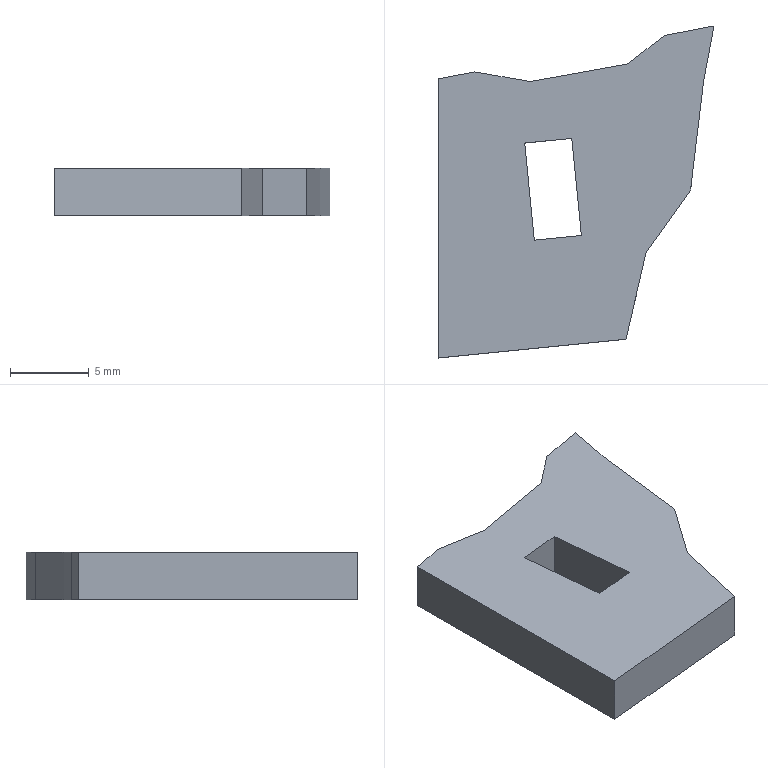Part | SolidWorks | features BaseBody 1 | 1 solid | 17 faces | box 17.508 x 21.063 x 3 mm | volume 743.607 mm3 | spline 10 | plane 7
STEP:
#1=CARTESIAN_POINT('',(4.82,4.837,-1.5));
#2=VERTEX_POINT('',#1);
#3=CARTESIAN_POINT('',(5.43,-1.324,-1.5));
#4=VERTEX_POINT('',#3);
#5=CARTESIAN_POINT('',(5.43,-1.324,-1.5));
#6=DIRECTION('',(0.09851,-0.9951,0.));
#7=VECTOR('',#6,1000.);
#8=LINE('',#5,#7);
#9=EDGE_CURVE('',#2,#4,#8,.T.);
#10=ORIENTED_EDGE('',*,*,#9,.F.);
#11=CARTESIAN_POINT('',(4.82,4.837,1.5));
#12=VERTEX_POINT('',#11);
#13=CARTESIAN_POINT('',(4.82,4.837,1.5));
#14=DIRECTION('',(0.,0.,-1.));
#15=VECTOR('',#14,1000.);
#16=LINE('',#13,#15);
#17=EDGE_CURVE('',#12,#2,#16,.T.);
#18=ORIENTED_EDGE('',*,*,#17,.F.);
#19=CARTESIAN_POINT('',(5.43,-1.324,1.5));
#20=VERTEX_POINT('',#19);
#21=CARTESIAN_POINT('',(5.43,-1.324,1.5));
#22=DIRECTION('',(0.09851,-0.9951,0.));
#23=VECTOR('',#22,1000.);
#24=LINE('',#21,#23);
#25=EDGE_CURVE('',#12,#20,#24,.T.);
#26=ORIENTED_EDGE('',*,*,#25,.T.);
#27=CARTESIAN_POINT('',(5.43,-1.324,1.5));
#28=DIRECTION('',(0.,0.,-1.));
#29=VECTOR('',#28,1000.);
#30=LINE('',#27,#29);
#31=EDGE_CURVE('',#20,#4,#30,.T.);
#32=ORIENTED_EDGE('',*,*,#31,.T.);
#33=EDGE_LOOP('',(#10,#18,#26,#32));
#34=FACE_OUTER_BOUND('',#33,.T.);
#35=CARTESIAN_POINT('',(5.43,-1.324,1.5));
#36=DIRECTION('',(0.9951,0.09851,0.));
#37=DIRECTION('',(0.,0.,-1.));
#38=AXIS2_PLACEMENT_3D('',#35,#36,#37);
#39=PLANE('',#38);
#40=ADVANCED_FACE('',(#34),#39,.T.);
#41=CARTESIAN_POINT('',(7.805,5.132,-1.5));
#42=VERTEX_POINT('',#41);
#43=CARTESIAN_POINT('',(7.805,5.132,-1.5));
#44=DIRECTION('',(-0.9951,-0.09851,0.));
#45=VECTOR('',#44,1000.);
#46=LINE('',#43,#45);
#47=EDGE_CURVE('',#42,#2,#46,.T.);
#48=ORIENTED_EDGE('',*,*,#47,.F.);
#49=CARTESIAN_POINT('',(7.805,5.132,1.5));
#50=VERTEX_POINT('',#49);
#51=CARTESIAN_POINT('',(7.805,5.132,1.5));
#52=DIRECTION('',(0.,0.,-1.));
#53=VECTOR('',#52,1000.);
#54=LINE('',#51,#53);
#55=EDGE_CURVE('',#50,#42,#54,.T.);
#56=ORIENTED_EDGE('',*,*,#55,.F.);
#57=CARTESIAN_POINT('',(7.805,5.132,1.5));
#58=DIRECTION('',(-0.9951,-0.09851,0.));
#59=VECTOR('',#58,1000.);
#60=LINE('',#57,#59);
#61=EDGE_CURVE('',#50,#12,#60,.T.);
#62=ORIENTED_EDGE('',*,*,#61,.T.);
#63=ORIENTED_EDGE('',*,*,#17,.T.);
#64=EDGE_LOOP('',(#48,#56,#62,#63));
#65=FACE_OUTER_BOUND('',#64,.T.);
#66=CARTESIAN_POINT('',(7.805,5.132,1.5));
#67=DIRECTION('',(0.09851,-0.9951,0.));
#68=DIRECTION('',(0.,0.,-1.));
#69=AXIS2_PLACEMENT_3D('',#66,#67,#68);
#70=PLANE('',#69);
#71=ADVANCED_FACE('',(#65),#70,.T.);
#72=CARTESIAN_POINT('',(8.415,-1.029,-1.5));
#73=VERTEX_POINT('',#72);
#74=CARTESIAN_POINT('',(8.415,-1.029,-1.5));
#75=DIRECTION('',(-0.09851,0.9951,0.));
#76=VECTOR('',#75,1000.);
#77=LINE('',#74,#76);
#78=EDGE_CURVE('',#73,#42,#77,.T.);
#79=ORIENTED_EDGE('',*,*,#78,.F.);
#80=CARTESIAN_POINT('',(8.415,-1.029,1.5));
#81=VERTEX_POINT('',#80);
#82=CARTESIAN_POINT('',(8.415,-1.029,1.5));
#83=DIRECTION('',(0.,0.,-1.));
#84=VECTOR('',#83,1000.);
#85=LINE('',#82,#84);
#86=EDGE_CURVE('',#81,#73,#85,.T.);
#87=ORIENTED_EDGE('',*,*,#86,.F.);
#88=CARTESIAN_POINT('',(8.415,-1.029,1.5));
#89=DIRECTION('',(-0.09851,0.9951,0.));
#90=VECTOR('',#89,1000.);
#91=LINE('',#88,#90);
#92=EDGE_CURVE('',#81,#50,#91,.T.);
#93=ORIENTED_EDGE('',*,*,#92,.T.);
#94=ORIENTED_EDGE('',*,*,#55,.T.);
#95=EDGE_LOOP('',(#79,#87,#93,#94));
#96=FACE_OUTER_BOUND('',#95,.T.);
#97=CARTESIAN_POINT('',(8.415,-1.029,1.5));
#98=DIRECTION('',(-0.9951,-0.09851,0.));
#99=DIRECTION('',(-0.09851,0.9951,0.));
#100=AXIS2_PLACEMENT_3D('',#97,#98,#99);
#101=PLANE('',#100);
#102=ADVANCED_FACE('',(#96),#101,.T.);
#103=CARTESIAN_POINT('',(8.415,-1.029,-1.5));
#104=DIRECTION('',(0.9951,0.09851,0.));
#105=VECTOR('',#104,1000.);
#106=LINE('',#103,#105);
#107=EDGE_CURVE('',#4,#73,#106,.T.);
#108=ORIENTED_EDGE('',*,*,#107,.F.);
#109=ORIENTED_EDGE('',*,*,#31,.F.);
#110=CARTESIAN_POINT('',(8.415,-1.029,1.5));
#111=DIRECTION('',(0.9951,0.09851,0.));
#112=VECTOR('',#111,1000.);
#113=LINE('',#110,#112);
#114=EDGE_CURVE('',#20,#81,#113,.T.);
#115=ORIENTED_EDGE('',*,*,#114,.T.);
#116=ORIENTED_EDGE('',*,*,#86,.T.);
#117=EDGE_LOOP('',(#108,#109,#115,#116));
#118=FACE_OUTER_BOUND('',#117,.T.);
#119=CARTESIAN_POINT('',(8.415,-1.029,1.5));
#120=DIRECTION('',(-0.09851,0.9951,0.));
#121=DIRECTION('',(0.,0.,1.));
#122=AXIS2_PLACEMENT_3D('',#119,#120,#121);
#123=PLANE('',#122);
#124=ADVANCED_FACE('',(#118),#123,.T.);
#125=CARTESIAN_POINT('',(5.187,8.742,-1.5));
#126=VERTEX_POINT('',#125);
#127=CARTESIAN_POINT('',(1.634,9.355,-1.5));
#128=VERTEX_POINT('',#127);
#129=CARTESIAN_POINT('',(5.187,8.742,-1.5));
#130=CARTESIAN_POINT('',(4.001,8.946,-1.5));
#131=CARTESIAN_POINT('',(2.817,9.149,-1.5));
#132=CARTESIAN_POINT('',(1.634,9.355,-1.5));
#133=B_SPLINE_CURVE_WITH_KNOTS('',3,(#129,#130,#131,#132),.UNSPECIFIED.,.F.,.F.,(4,4),(0.5238,0.5714),.UNSPECIFIED.);
#134=EDGE_CURVE('',#126,#128,#133,.T.);
#135=ORIENTED_EDGE('',*,*,#134,.T.);
#136=CARTESIAN_POINT('',(1.634,9.355,1.5));
#137=VERTEX_POINT('',#136);
#138=CARTESIAN_POINT('',(1.634,9.355,1.5));
#139=DIRECTION('',(0.,0.,-1.));
#140=VECTOR('',#139,1000.);
#141=LINE('',#138,#140);
#142=EDGE_CURVE('',#137,#128,#141,.T.);
#143=ORIENTED_EDGE('',*,*,#142,.F.);
#144=CARTESIAN_POINT('',(5.187,8.742,1.5));
#145=VERTEX_POINT('',#144);
#146=CARTESIAN_POINT('',(5.187,8.742,1.5));
#147=CARTESIAN_POINT('',(4.001,8.946,1.5));
#148=CARTESIAN_POINT('',(2.817,9.149,1.5));
#149=CARTESIAN_POINT('',(1.634,9.355,1.5));
#150=B_SPLINE_CURVE_WITH_KNOTS('',3,(#146,#147,#148,#149),.UNSPECIFIED.,.F.,.F.,(4,4),(0.5238,0.5714),.UNSPECIFIED.);
#151=EDGE_CURVE('',#145,#137,#150,.T.);
#152=ORIENTED_EDGE('',*,*,#151,.F.);
#153=CARTESIAN_POINT('',(5.187,8.742,1.5));
#154=DIRECTION('',(0.,0.,-1.));
#155=VECTOR('',#154,1000.);
#156=LINE('',#153,#155);
#157=EDGE_CURVE('',#145,#126,#156,.T.);
#158=ORIENTED_EDGE('',*,*,#157,.T.);
#159=EDGE_LOOP('',(#135,#143,#152,#158));
#160=FACE_OUTER_BOUND('',#159,.T.);
#161=CARTESIAN_POINT('',(5.187,8.742,1.5));
#162=CARTESIAN_POINT('',(5.187,8.742,-1.5));
#163=CARTESIAN_POINT('',(4.001,8.946,1.5));
#164=CARTESIAN_POINT('',(4.001,8.946,-1.5));
#165=CARTESIAN_POINT('',(2.817,9.149,1.5));
#166=CARTESIAN_POINT('',(2.817,9.149,-1.5));
#167=CARTESIAN_POINT('',(1.634,9.355,1.5));
#168=CARTESIAN_POINT('',(1.634,9.355,-1.5));
#169=B_SPLINE_SURFACE_WITH_KNOTS('',3,1,((#161,#162),(#163,#164),(#165,#166),(#167,#168)),.UNSPECIFIED.,.F.,.F.,.F.,(4,4),(2,2),(0.5238,0.5714),(0.,1.),.UNSPECIFIED.);
#170=ADVANCED_FACE('',(#160),#169,.F.);
#171=CARTESIAN_POINT('',(11.344,9.856,-1.5));
#172=VERTEX_POINT('',#171);
#173=CARTESIAN_POINT('',(11.344,9.856,-1.5));
#174=CARTESIAN_POINT('',(9.29,9.485,-1.5));
#175=CARTESIAN_POINT('',(7.239,9.113,-1.5));
#176=CARTESIAN_POINT('',(5.187,8.742,-1.5));
#177=B_SPLINE_CURVE_WITH_KNOTS('',3,(#173,#174,#175,#176),.UNSPECIFIED.,.F.,.F.,(4,4),(0.5714,0.619),.UNSPECIFIED.);
#178=EDGE_CURVE('',#172,#126,#177,.T.);
#179=ORIENTED_EDGE('',*,*,#178,.T.);
#180=ORIENTED_EDGE('',*,*,#157,.F.);
#181=CARTESIAN_POINT('',(11.344,9.856,1.5));
#182=VERTEX_POINT('',#181);
#183=CARTESIAN_POINT('',(11.344,9.856,1.5));
#184=CARTESIAN_POINT('',(9.29,9.485,1.5));
#185=CARTESIAN_POINT('',(7.239,9.113,1.5));
#186=CARTESIAN_POINT('',(5.187,8.742,1.5));
#187=B_SPLINE_CURVE_WITH_KNOTS('',3,(#183,#184,#185,#186),.UNSPECIFIED.,.F.,.F.,(4,4),(0.5714,0.619),.UNSPECIFIED.);
#188=EDGE_CURVE('',#182,#145,#187,.T.);
#189=ORIENTED_EDGE('',*,*,#188,.F.);
#190=CARTESIAN_POINT('',(11.344,9.856,1.5));
#191=DIRECTION('',(0.,0.,-1.));
#192=VECTOR('',#191,1000.);
#193=LINE('',#190,#192);
#194=EDGE_CURVE('',#182,#172,#193,.T.);
#195=ORIENTED_EDGE('',*,*,#194,.T.);
#196=EDGE_LOOP('',(#179,#180,#189,#195));
#197=FACE_OUTER_BOUND('',#196,.T.);
#198=CARTESIAN_POINT('',(11.344,9.856,1.5));
#199=CARTESIAN_POINT('',(11.344,9.856,-1.5));
#200=CARTESIAN_POINT('',(9.29,9.485,1.5));
#201=CARTESIAN_POINT('',(9.29,9.485,-1.5));
#202=CARTESIAN_POINT('',(7.239,9.113,1.5));
#203=CARTESIAN_POINT('',(7.239,9.113,-1.5));
#204=CARTESIAN_POINT('',(5.187,8.742,1.5));
#205=CARTESIAN_POINT('',(5.187,8.742,-1.5));
#206=B_SPLINE_SURFACE_WITH_KNOTS('',3,1,((#198,#199),(#200,#201),(#202,#203),(#204,#205)),.UNSPECIFIED.,.F.,.F.,.F.,(4,4),(2,2),(0.5714,0.619),(0.,1.),.UNSPECIFIED.);
#207=ADVANCED_FACE('',(#197),#206,.F.);
#208=CARTESIAN_POINT('',(13.682,11.663,-1.5));
#209=VERTEX_POINT('',#208);
#210=CARTESIAN_POINT('',(13.682,11.663,-1.5));
#211=CARTESIAN_POINT('',(12.903,11.062,-1.5));
#212=CARTESIAN_POINT('',(12.123,10.459,-1.5));
#213=CARTESIAN_POINT('',(11.344,9.856,-1.5));
#214=B_SPLINE_CURVE_WITH_KNOTS('',3,(#210,#211,#212,#213),.UNSPECIFIED.,.F.,.F.,(4,4),(0.619,0.6667),.UNSPECIFIED.);
#215=EDGE_CURVE('',#209,#172,#214,.T.);
#216=ORIENTED_EDGE('',*,*,#215,.T.);
#217=ORIENTED_EDGE('',*,*,#194,.F.);
#218=CARTESIAN_POINT('',(13.682,11.663,1.5));
#219=VERTEX_POINT('',#218);
#220=CARTESIAN_POINT('',(13.682,11.663,1.5));
#221=CARTESIAN_POINT('',(12.903,11.062,1.5));
#222=CARTESIAN_POINT('',(12.123,10.459,1.5));
#223=CARTESIAN_POINT('',(11.344,9.856,1.5));
#224=B_SPLINE_CURVE_WITH_KNOTS('',3,(#220,#221,#222,#223),.UNSPECIFIED.,.F.,.F.,(4,4),(0.619,0.6667),.UNSPECIFIED.);
#225=EDGE_CURVE('',#219,#182,#224,.T.);
#226=ORIENTED_EDGE('',*,*,#225,.F.);
#227=CARTESIAN_POINT('',(13.682,11.663,1.5));
#228=DIRECTION('',(0.,0.,-1.));
#229=VECTOR('',#228,1000.);
#230=LINE('',#227,#229);
#231=EDGE_CURVE('',#219,#209,#230,.T.);
#232=ORIENTED_EDGE('',*,*,#231,.T.);
#233=EDGE_LOOP('',(#216,#217,#226,#232));
#234=FACE_OUTER_BOUND('',#233,.T.);
#235=CARTESIAN_POINT('',(13.682,11.663,1.5));
#236=CARTESIAN_POINT('',(13.682,11.663,-1.5));
#237=CARTESIAN_POINT('',(12.903,11.062,1.5));
#238=CARTESIAN_POINT('',(12.903,11.062,-1.5));
#239=CARTESIAN_POINT('',(12.123,10.459,1.5));
#240=CARTESIAN_POINT('',(12.123,10.459,-1.5));
#241=CARTESIAN_POINT('',(11.344,9.856,1.5));
#242=CARTESIAN_POINT('',(11.344,9.856,-1.5));
#243=B_SPLINE_SURFACE_WITH_KNOTS('',3,1,((#235,#236),(#237,#238),(#239,#240),(#241,#242)),.UNSPECIFIED.,.F.,.F.,.F.,(4,4),(2,2),(0.619,0.6667),(0.,1.),.UNSPECIFIED.);
#244=ADVANCED_FACE('',(#234),#243,.F.);
#245=CARTESIAN_POINT('',(16.827,12.266,-1.5));
#246=VERTEX_POINT('',#245);
#247=CARTESIAN_POINT('',(16.827,12.266,-1.5));
#248=CARTESIAN_POINT('',(15.779,12.065,-1.5));
#249=CARTESIAN_POINT('',(14.73,11.862,-1.5));
#250=CARTESIAN_POINT('',(13.682,11.663,-1.5));
#251=B_SPLINE_CURVE_WITH_KNOTS('',3,(#247,#248,#249,#250),.UNSPECIFIED.,.F.,.F.,(4,4),(0.6667,0.7143),.UNSPECIFIED.);
#252=EDGE_CURVE('',#246,#209,#251,.T.);
#253=ORIENTED_EDGE('',*,*,#252,.T.);
#254=ORIENTED_EDGE('',*,*,#231,.F.);
#255=CARTESIAN_POINT('',(16.827,12.266,1.5));
#256=VERTEX_POINT('',#255);
#257=CARTESIAN_POINT('',(16.827,12.266,1.5));
#258=CARTESIAN_POINT('',(15.779,12.065,1.5));
#259=CARTESIAN_POINT('',(14.73,11.862,1.5));
#260=CARTESIAN_POINT('',(13.682,11.663,1.5));
#261=B_SPLINE_CURVE_WITH_KNOTS('',3,(#257,#258,#259,#260),.UNSPECIFIED.,.F.,.F.,(4,4),(0.6667,0.7143),.UNSPECIFIED.);
#262=EDGE_CURVE('',#256,#219,#261,.T.);
#263=ORIENTED_EDGE('',*,*,#262,.F.);
#264=CARTESIAN_POINT('',(16.827,12.266,1.5));
#265=DIRECTION('',(0.,0.,-1.));
#266=VECTOR('',#265,1000.);
#267=LINE('',#264,#266);
#268=EDGE_CURVE('',#256,#246,#267,.T.);
#269=ORIENTED_EDGE('',*,*,#268,.T.);
#270=EDGE_LOOP('',(#253,#254,#263,#269));
#271=FACE_OUTER_BOUND('',#270,.T.);
#272=CARTESIAN_POINT('',(16.827,12.266,1.5));
#273=CARTESIAN_POINT('',(16.827,12.266,-1.5));
#274=CARTESIAN_POINT('',(15.779,12.065,1.5));
#275=CARTESIAN_POINT('',(15.779,12.065,-1.5));
#276=CARTESIAN_POINT('',(14.73,11.862,1.5));
#277=CARTESIAN_POINT('',(14.73,11.862,-1.5));
#278=CARTESIAN_POINT('',(13.682,11.663,1.5));
#279=CARTESIAN_POINT('',(13.682,11.663,-1.5));
#280=B_SPLINE_SURFACE_WITH_KNOTS('',3,1,((#272,#273),(#274,#275),(#276,#277),(#278,#279)),.UNSPECIFIED.,.F.,.F.,.F.,(4,4),(2,2),(0.6667,0.7143),(0.,1.),.UNSPECIFIED.);
#281=ADVANCED_FACE('',(#271),#280,.F.);
#282=CARTESIAN_POINT('',(16.177,8.839,-1.5));
#283=VERTEX_POINT('',#282);
#284=CARTESIAN_POINT('',(16.177,8.839,-1.5));
#285=CARTESIAN_POINT('',(16.394,9.981,-1.5));
#286=CARTESIAN_POINT('',(16.612,11.122,-1.5));
#287=CARTESIAN_POINT('',(16.827,12.266,-1.5));
#288=B_SPLINE_CURVE_WITH_KNOTS('',3,(#284,#285,#286,#287),.UNSPECIFIED.,.F.,.F.,(4,4),(0.7143,0.7619),.UNSPECIFIED.);
#289=EDGE_CURVE('',#283,#246,#288,.T.);
#290=ORIENTED_EDGE('',*,*,#289,.T.);
#291=ORIENTED_EDGE('',*,*,#268,.F.);
#292=CARTESIAN_POINT('',(16.177,8.839,1.5));
#293=VERTEX_POINT('',#292);
#294=CARTESIAN_POINT('',(16.177,8.839,1.5));
#295=CARTESIAN_POINT('',(16.394,9.981,1.5));
#296=CARTESIAN_POINT('',(16.612,11.122,1.5));
#297=CARTESIAN_POINT('',(16.827,12.266,1.5));
#298=B_SPLINE_CURVE_WITH_KNOTS('',3,(#294,#295,#296,#297),.UNSPECIFIED.,.F.,.F.,(4,4),(0.7143,0.7619),.UNSPECIFIED.);
#299=EDGE_CURVE('',#293,#256,#298,.T.);
#300=ORIENTED_EDGE('',*,*,#299,.F.);
#301=CARTESIAN_POINT('',(16.177,8.839,1.5));
#302=DIRECTION('',(0.,0.,-1.));
#303=VECTOR('',#302,1000.);
#304=LINE('',#301,#303);
#305=EDGE_CURVE('',#293,#283,#304,.T.);
#306=ORIENTED_EDGE('',*,*,#305,.T.);
#307=EDGE_LOOP('',(#290,#291,#300,#306));
#308=FACE_OUTER_BOUND('',#307,.T.);
#309=CARTESIAN_POINT('',(16.177,8.839,1.5));
#310=CARTESIAN_POINT('',(16.177,8.839,-1.5));
#311=CARTESIAN_POINT('',(16.394,9.981,1.5));
#312=CARTESIAN_POINT('',(16.394,9.981,-1.5));
#313=CARTESIAN_POINT('',(16.612,11.122,1.5));
#314=CARTESIAN_POINT('',(16.612,11.122,-1.5));
#315=CARTESIAN_POINT('',(16.827,12.266,1.5));
#316=CARTESIAN_POINT('',(16.827,12.266,-1.5));
#317=B_SPLINE_SURFACE_WITH_KNOTS('',3,1,((#309,#310),(#311,#312),(#313,#314),(#315,#316)),.UNSPECIFIED.,.F.,.F.,.F.,(4,4),(2,2),(0.7143,0.7619),(0.,1.),.UNSPECIFIED.);
#318=ADVANCED_FACE('',(#308),#317,.F.);
#319=CARTESIAN_POINT('',(15.344,1.858,-1.5));
#320=VERTEX_POINT('',#319);
#321=CARTESIAN_POINT('',(15.344,1.858,-1.5));
#322=CARTESIAN_POINT('',(15.623,4.185,-1.5));
#323=CARTESIAN_POINT('',(15.902,6.512,-1.5));
#324=CARTESIAN_POINT('',(16.177,8.839,-1.5));
#325=B_SPLINE_CURVE_WITH_KNOTS('',3,(#321,#322,#323,#324),.UNSPECIFIED.,.F.,.F.,(4,4),(0.7619,0.8095),.UNSPECIFIED.);
#326=EDGE_CURVE('',#320,#283,#325,.T.);
#327=ORIENTED_EDGE('',*,*,#326,.T.);
#328=ORIENTED_EDGE('',*,*,#305,.F.);
#329=CARTESIAN_POINT('',(15.344,1.858,1.5));
#330=VERTEX_POINT('',#329);
#331=CARTESIAN_POINT('',(15.344,1.858,1.5));
#332=CARTESIAN_POINT('',(15.623,4.185,1.5));
#333=CARTESIAN_POINT('',(15.902,6.512,1.5));
#334=CARTESIAN_POINT('',(16.177,8.839,1.5));
#335=B_SPLINE_CURVE_WITH_KNOTS('',3,(#331,#332,#333,#334),.UNSPECIFIED.,.F.,.F.,(4,4),(0.7619,0.8095),.UNSPECIFIED.);
#336=EDGE_CURVE('',#330,#293,#335,.T.);
#337=ORIENTED_EDGE('',*,*,#336,.F.);
#338=CARTESIAN_POINT('',(15.344,1.858,1.5));
#339=DIRECTION('',(0.,0.,-1.));
#340=VECTOR('',#339,1000.);
#341=LINE('',#338,#340);
#342=EDGE_CURVE('',#330,#320,#341,.T.);
#343=ORIENTED_EDGE('',*,*,#342,.T.);
#344=EDGE_LOOP('',(#327,#328,#337,#343));
#345=FACE_OUTER_BOUND('',#344,.T.);
#346=CARTESIAN_POINT('',(15.344,1.858,1.5));
#347=CARTESIAN_POINT('',(15.344,1.858,-1.5));
#348=CARTESIAN_POINT('',(15.623,4.185,1.5));
#349=CARTESIAN_POINT('',(15.623,4.185,-1.5));
#350=CARTESIAN_POINT('',(15.902,6.512,1.5));
#351=CARTESIAN_POINT('',(15.902,6.512,-1.5));
#352=CARTESIAN_POINT('',(16.177,8.839,1.5));
#353=CARTESIAN_POINT('',(16.177,8.839,-1.5));
#354=B_SPLINE_SURFACE_WITH_KNOTS('',3,1,((#346,#347),(#348,#349),(#350,#351),(#352,#353)),.UNSPECIFIED.,.F.,.F.,.F.,(4,4),(2,2),(0.7619,0.8095),(0.,1.),.UNSPECIFIED.);
#355=ADVANCED_FACE('',(#345),#354,.F.);
#356=CARTESIAN_POINT('',(12.521,-2.113,-1.5));
#357=VERTEX_POINT('',#356);
#358=CARTESIAN_POINT('',(12.521,-2.113,-1.5));
#359=CARTESIAN_POINT('',(13.464,-0.7892,-1.5));
#360=CARTESIAN_POINT('',(14.405,0.5349,-1.5));
#361=CARTESIAN_POINT('',(15.344,1.858,-1.5));
#362=B_SPLINE_CURVE_WITH_KNOTS('',3,(#358,#359,#360,#361),.UNSPECIFIED.,.F.,.F.,(4,4),(0.8095,0.8571),.UNSPECIFIED.);
#363=EDGE_CURVE('',#357,#320,#362,.T.);
#364=ORIENTED_EDGE('',*,*,#363,.T.);
#365=ORIENTED_EDGE('',*,*,#342,.F.);
#366=CARTESIAN_POINT('',(12.521,-2.113,1.5));
#367=VERTEX_POINT('',#366);
#368=CARTESIAN_POINT('',(12.521,-2.113,1.5));
#369=CARTESIAN_POINT('',(13.464,-0.7892,1.5));
#370=CARTESIAN_POINT('',(14.405,0.5349,1.5));
#371=CARTESIAN_POINT('',(15.344,1.858,1.5));
#372=B_SPLINE_CURVE_WITH_KNOTS('',3,(#368,#369,#370,#371),.UNSPECIFIED.,.F.,.F.,(4,4),(0.8095,0.8571),.UNSPECIFIED.);
#373=EDGE_CURVE('',#367,#330,#372,.T.);
#374=ORIENTED_EDGE('',*,*,#373,.F.);
#375=CARTESIAN_POINT('',(12.521,-2.113,1.5));
#376=DIRECTION('',(0.,0.,-1.));
#377=VECTOR('',#376,1000.);
#378=LINE('',#375,#377);
#379=EDGE_CURVE('',#367,#357,#378,.T.);
#380=ORIENTED_EDGE('',*,*,#379,.T.);
#381=EDGE_LOOP('',(#364,#365,#374,#380));
#382=FACE_OUTER_BOUND('',#381,.T.);
#383=CARTESIAN_POINT('',(12.521,-2.113,1.5));
#384=CARTESIAN_POINT('',(12.521,-2.113,-1.5));
#385=CARTESIAN_POINT('',(13.464,-0.7892,1.5));
#386=CARTESIAN_POINT('',(13.464,-0.7892,-1.5));
#387=CARTESIAN_POINT('',(14.405,0.5349,1.5));
#388=CARTESIAN_POINT('',(14.405,0.5349,-1.5));
#389=CARTESIAN_POINT('',(15.344,1.858,1.5));
#390=CARTESIAN_POINT('',(15.344,1.858,-1.5));
#391=B_SPLINE_SURFACE_WITH_KNOTS('',3,1,((#383,#384),(#385,#386),(#387,#388),(#389,#390)),.UNSPECIFIED.,.F.,.F.,.F.,(4,4),(2,2),(0.8095,0.8571),(0.,1.),.UNSPECIFIED.);
#392=ADVANCED_FACE('',(#382),#391,.F.);
#393=CARTESIAN_POINT('',(11.243,-7.615,-1.5));
#394=VERTEX_POINT('',#393);
#395=CARTESIAN_POINT('',(11.243,-7.615,-1.5));
#396=CARTESIAN_POINT('',(11.669,-5.78,-1.5));
#397=CARTESIAN_POINT('',(12.097,-3.948,-1.5));
#398=CARTESIAN_POINT('',(12.521,-2.113,-1.5));
#399=B_SPLINE_CURVE_WITH_KNOTS('',3,(#395,#396,#397,#398),.UNSPECIFIED.,.F.,.F.,(4,4),(0.8571,0.9048),.UNSPECIFIED.);
#400=EDGE_CURVE('',#394,#357,#399,.T.);
#401=ORIENTED_EDGE('',*,*,#400,.T.);
#402=ORIENTED_EDGE('',*,*,#379,.F.);
#403=CARTESIAN_POINT('',(11.243,-7.615,1.5));
#404=VERTEX_POINT('',#403);
#405=CARTESIAN_POINT('',(11.243,-7.615,1.5));
#406=CARTESIAN_POINT('',(11.669,-5.78,1.5));
#407=CARTESIAN_POINT('',(12.097,-3.948,1.5));
#408=CARTESIAN_POINT('',(12.521,-2.113,1.5));
#409=B_SPLINE_CURVE_WITH_KNOTS('',3,(#405,#406,#407,#408),.UNSPECIFIED.,.F.,.F.,(4,4),(0.8571,0.9048),.UNSPECIFIED.);
#410=EDGE_CURVE('',#404,#367,#409,.T.);
#411=ORIENTED_EDGE('',*,*,#410,.F.);
#412=CARTESIAN_POINT('',(11.243,-7.615,1.5));
#413=DIRECTION('',(0.,0.,-1.));
#414=VECTOR('',#413,1000.);
#415=LINE('',#412,#414);
#416=EDGE_CURVE('',#404,#394,#415,.T.);
#417=ORIENTED_EDGE('',*,*,#416,.T.);
#418=EDGE_LOOP('',(#401,#402,#411,#417));
#419=FACE_OUTER_BOUND('',#418,.T.);
#420=CARTESIAN_POINT('',(11.243,-7.615,1.5));
#421=CARTESIAN_POINT('',(11.243,-7.615,-1.5));
#422=CARTESIAN_POINT('',(11.669,-5.78,1.5));
#423=CARTESIAN_POINT('',(11.669,-5.78,-1.5));
#424=CARTESIAN_POINT('',(12.097,-3.948,1.5));
#425=CARTESIAN_POINT('',(12.097,-3.948,-1.5));
#426=CARTESIAN_POINT('',(12.521,-2.113,1.5));
#427=CARTESIAN_POINT('',(12.521,-2.113,-1.5));
#428=B_SPLINE_SURFACE_WITH_KNOTS('',3,1,((#420,#421),(#422,#423),(#424,#425),(#426,#427)),.UNSPECIFIED.,.F.,.F.,.F.,(4,4),(2,2),(0.8571,0.9048),(0.,1.),.UNSPECIFIED.);
#429=ADVANCED_FACE('',(#419),#428,.F.);
#430=CARTESIAN_POINT('',(-0.6806,-8.797,-1.5));
#431=VERTEX_POINT('',#430);
#432=CARTESIAN_POINT('',(-0.6806,-8.797,-1.5));
#433=CARTESIAN_POINT('',(3.294,-8.402,-1.5));
#434=CARTESIAN_POINT('',(7.27,-8.009,-1.5));
#435=CARTESIAN_POINT('',(11.243,-7.615,-1.5));
#436=B_SPLINE_CURVE_WITH_KNOTS('',3,(#432,#433,#434,#435),.UNSPECIFIED.,.F.,.F.,(4,4),(0.9048,1.),.UNSPECIFIED.);
#437=EDGE_CURVE('',#431,#394,#436,.T.);
#438=ORIENTED_EDGE('',*,*,#437,.T.);
#439=ORIENTED_EDGE('',*,*,#416,.F.);
#440=CARTESIAN_POINT('',(-0.6806,-8.797,1.5));
#441=VERTEX_POINT('',#440);
#442=CARTESIAN_POINT('',(-0.6806,-8.797,1.5));
#443=CARTESIAN_POINT('',(3.294,-8.402,1.5));
#444=CARTESIAN_POINT('',(7.27,-8.009,1.5));
#445=CARTESIAN_POINT('',(11.243,-7.615,1.5));
#446=B_SPLINE_CURVE_WITH_KNOTS('',3,(#442,#443,#444,#445),.UNSPECIFIED.,.F.,.F.,(4,4),(0.9048,1.),.UNSPECIFIED.);
#447=EDGE_CURVE('',#441,#404,#446,.T.);
#448=ORIENTED_EDGE('',*,*,#447,.F.);
#449=CARTESIAN_POINT('',(-0.6806,-8.797,1.5));
#450=DIRECTION('',(0.,0.,-1.));
#451=VECTOR('',#450,1000.);
#452=LINE('',#449,#451);
#453=EDGE_CURVE('',#441,#431,#452,.T.);
#454=ORIENTED_EDGE('',*,*,#453,.T.);
#455=EDGE_LOOP('',(#438,#439,#448,#454));
#456=FACE_OUTER_BOUND('',#455,.T.);
#457=CARTESIAN_POINT('',(-0.6806,-8.797,1.5));
#458=CARTESIAN_POINT('',(-0.6806,-8.797,-1.5));
#459=CARTESIAN_POINT('',(3.294,-8.402,1.5));
#460=CARTESIAN_POINT('',(3.294,-8.402,-1.5));
#461=CARTESIAN_POINT('',(7.27,-8.009,1.5));
#462=CARTESIAN_POINT('',(7.27,-8.009,-1.5));
#463=CARTESIAN_POINT('',(11.243,-7.615,1.5));
#464=CARTESIAN_POINT('',(11.243,-7.615,-1.5));
#465=B_SPLINE_SURFACE_WITH_KNOTS('',3,1,((#457,#458),(#459,#460),(#461,#462),(#463,#464)),.UNSPECIFIED.,.F.,.F.,.F.,(4,4),(2,2),(0.9048,1.),(0.,1.),.UNSPECIFIED.);
#466=ADVANCED_FACE('',(#456),#465,.F.);
#467=CARTESIAN_POINT('',(-0.6806,8.91,-1.5));
#468=VERTEX_POINT('',#467);
#469=CARTESIAN_POINT('',(-0.6806,8.91,-1.5));
#470=DIRECTION('',(0.,-1.,0.));
#471=VECTOR('',#470,1000.);
#472=LINE('',#469,#471);
#473=EDGE_CURVE('',#468,#431,#472,.T.);
#474=ORIENTED_EDGE('',*,*,#473,.T.);
#475=ORIENTED_EDGE('',*,*,#453,.F.);
#476=CARTESIAN_POINT('',(-0.6806,8.91,1.5));
#477=VERTEX_POINT('',#476);
#478=CARTESIAN_POINT('',(-0.6806,8.91,1.5));
#479=DIRECTION('',(0.,-1.,0.));
#480=VECTOR('',#479,1000.);
#481=LINE('',#478,#480);
#482=EDGE_CURVE('',#477,#441,#481,.T.);
#483=ORIENTED_EDGE('',*,*,#482,.F.);
#484=CARTESIAN_POINT('',(-0.6806,8.91,1.5));
#485=DIRECTION('',(0.,0.,-1.));
#486=VECTOR('',#485,1000.);
#487=LINE('',#484,#486);
#488=EDGE_CURVE('',#477,#468,#487,.T.);
#489=ORIENTED_EDGE('',*,*,#488,.T.);
#490=EDGE_LOOP('',(#474,#475,#483,#489));
#491=FACE_OUTER_BOUND('',#490,.T.);
#492=CARTESIAN_POINT('',(-0.6806,8.91,1.5));
#493=DIRECTION('',(1.,0.,0.));
#494=DIRECTION('',(0.,1.,0.));
#495=AXIS2_PLACEMENT_3D('',#492,#493,#494);
#496=PLANE('',#495);
#497=ADVANCED_FACE('',(#491),#496,.F.);
#498=CARTESIAN_POINT('',(1.634,9.355,-1.5));
#499=CARTESIAN_POINT('',(0.863,9.206,-1.5));
#500=CARTESIAN_POINT('',(0.09044,9.059,-1.5));
#501=CARTESIAN_POINT('',(-0.6806,8.91,-1.5));
#502=B_SPLINE_CURVE_WITH_KNOTS('',3,(#498,#499,#500,#501),.UNSPECIFIED.,.F.,.F.,(4,4),(0.4762,0.5238),.UNSPECIFIED.);
#503=EDGE_CURVE('',#128,#468,#502,.T.);
#504=ORIENTED_EDGE('',*,*,#503,.T.);
#505=ORIENTED_EDGE('',*,*,#488,.F.);
#506=CARTESIAN_POINT('',(1.634,9.355,1.5));
#507=CARTESIAN_POINT('',(0.863,9.206,1.5));
#508=CARTESIAN_POINT('',(0.09044,9.059,1.5));
#509=CARTESIAN_POINT('',(-0.6806,8.91,1.5));
#510=B_SPLINE_CURVE_WITH_KNOTS('',3,(#506,#507,#508,#509),.UNSPECIFIED.,.F.,.F.,(4,4),(0.4762,0.5238),.UNSPECIFIED.);
#511=EDGE_CURVE('',#137,#477,#510,.T.);
#512=ORIENTED_EDGE('',*,*,#511,.F.);
#513=ORIENTED_EDGE('',*,*,#142,.T.);
#514=EDGE_LOOP('',(#504,#505,#512,#513));
#515=FACE_OUTER_BOUND('',#514,.T.);
#516=CARTESIAN_POINT('',(1.634,9.355,1.5));
#517=CARTESIAN_POINT('',(1.634,9.355,-1.5));
#518=CARTESIAN_POINT('',(0.863,9.206,1.5));
#519=CARTESIAN_POINT('',(0.863,9.206,-1.5));
#520=CARTESIAN_POINT('',(0.09044,9.059,1.5));
#521=CARTESIAN_POINT('',(0.09044,9.059,-1.5));
#522=CARTESIAN_POINT('',(-0.6806,8.91,1.5));
#523=CARTESIAN_POINT('',(-0.6806,8.91,-1.5));
#524=B_SPLINE_SURFACE_WITH_KNOTS('',3,1,((#516,#517),(#518,#519),(#520,#521),(#522,#523)),.UNSPECIFIED.,.F.,.F.,.F.,(4,4),(2,2),(0.4762,0.5238),(0.,1.),.UNSPECIFIED.);
#525=ADVANCED_FACE('',(#515),#524,.F.);
#526=ORIENTED_EDGE('',*,*,#107,.T.);
#527=ORIENTED_EDGE('',*,*,#78,.T.);
#528=ORIENTED_EDGE('',*,*,#47,.T.);
#529=ORIENTED_EDGE('',*,*,#9,.T.);
#530=EDGE_LOOP('',(#526,#527,#528,#529));
#531=FACE_BOUND('',#530,.T.);
#532=ORIENTED_EDGE('',*,*,#503,.F.);
#533=ORIENTED_EDGE('',*,*,#134,.F.);
#534=ORIENTED_EDGE('',*,*,#178,.F.);
#535=ORIENTED_EDGE('',*,*,#215,.F.);
#536=ORIENTED_EDGE('',*,*,#252,.F.);
#537=ORIENTED_EDGE('',*,*,#289,.F.);
#538=ORIENTED_EDGE('',*,*,#326,.F.);
#539=ORIENTED_EDGE('',*,*,#363,.F.);
#540=ORIENTED_EDGE('',*,*,#400,.F.);
#541=ORIENTED_EDGE('',*,*,#437,.F.);
#542=ORIENTED_EDGE('',*,*,#473,.F.);
#543=EDGE_LOOP('',(#532,#533,#534,#535,#536,#537,#538,#539,#540,#541,#542));
#544=FACE_OUTER_BOUND('',#543,.T.);
#545=CARTESIAN_POINT('',(0.4767,9.133,-1.5));
#546=DIRECTION('',(0.,0.,1.));
#547=DIRECTION('',(1.,0.,0.));
#548=AXIS2_PLACEMENT_3D('',#545,#546,#547);
#549=PLANE('',#548);
#550=ADVANCED_FACE('',(#531,#544),#549,.F.);
#551=ORIENTED_EDGE('',*,*,#92,.F.);
#552=ORIENTED_EDGE('',*,*,#114,.F.);
#553=ORIENTED_EDGE('',*,*,#25,.F.);
#554=ORIENTED_EDGE('',*,*,#61,.F.);
#555=EDGE_LOOP('',(#551,#552,#553,#554));
#556=FACE_BOUND('',#555,.T.);
#557=ORIENTED_EDGE('',*,*,#511,.T.);
#558=ORIENTED_EDGE('',*,*,#482,.T.);
#559=ORIENTED_EDGE('',*,*,#447,.T.);
#560=ORIENTED_EDGE('',*,*,#410,.T.);
#561=ORIENTED_EDGE('',*,*,#373,.T.);
#562=ORIENTED_EDGE('',*,*,#336,.T.);
#563=ORIENTED_EDGE('',*,*,#299,.T.);
#564=ORIENTED_EDGE('',*,*,#262,.T.);
#565=ORIENTED_EDGE('',*,*,#225,.T.);
#566=ORIENTED_EDGE('',*,*,#188,.T.);
#567=ORIENTED_EDGE('',*,*,#151,.T.);
#568=EDGE_LOOP('',(#557,#558,#559,#560,#561,#562,#563,#564,#565,#566,#567));
#569=FACE_OUTER_BOUND('',#568,.T.);
#570=CARTESIAN_POINT('',(0.4767,9.133,1.5));
#571=DIRECTION('',(0.,0.,1.));
#572=DIRECTION('',(1.,0.,0.));
#573=AXIS2_PLACEMENT_3D('',#570,#571,#572);
#574=PLANE('',#573);
#575=ADVANCED_FACE('',(#556,#569),#574,.T.);
#576=CLOSED_SHELL('',(#40,#71,#102,#124,#170,#207,#244,#281,#318,#355,#392,#429,#466,#497,#525,#550,#575));
#577=MANIFOLD_SOLID_BREP('',#576);
#578=CARTESIAN_POINT('',(0.,0.,0.));
#579=DIRECTION('',(0.,0.,1.));
#580=DIRECTION('',(1.,0.,0.));
#581=AXIS2_PLACEMENT_3D('',#578,#579,#580);
#582=(LENGTH_UNIT()NAMED_UNIT(*)SI_UNIT(.MILLI.,.METRE.));
#583=UNCERTAINTY_MEASURE_WITH_UNIT(LENGTH_MEASURE(0.00001),#582,'','');
#584=(NAMED_UNIT(*)PLANE_ANGLE_UNIT()SI_UNIT($,.RADIAN.));
#585=(NAMED_UNIT(*)SI_UNIT($,.STERADIAN.)SOLID_ANGLE_UNIT());
#586=(GEOMETRIC_REPRESENTATION_CONTEXT(3)GLOBAL_UNCERTAINTY_ASSIGNED_CONTEXT((#583))GLOBAL_UNIT_ASSIGNED_CONTEXT((#582,#584,#585))REPRESENTATION_CONTEXT('',''));
#587=ADVANCED_BREP_SHAPE_REPRESENTATION('',(#577,#581),#586);